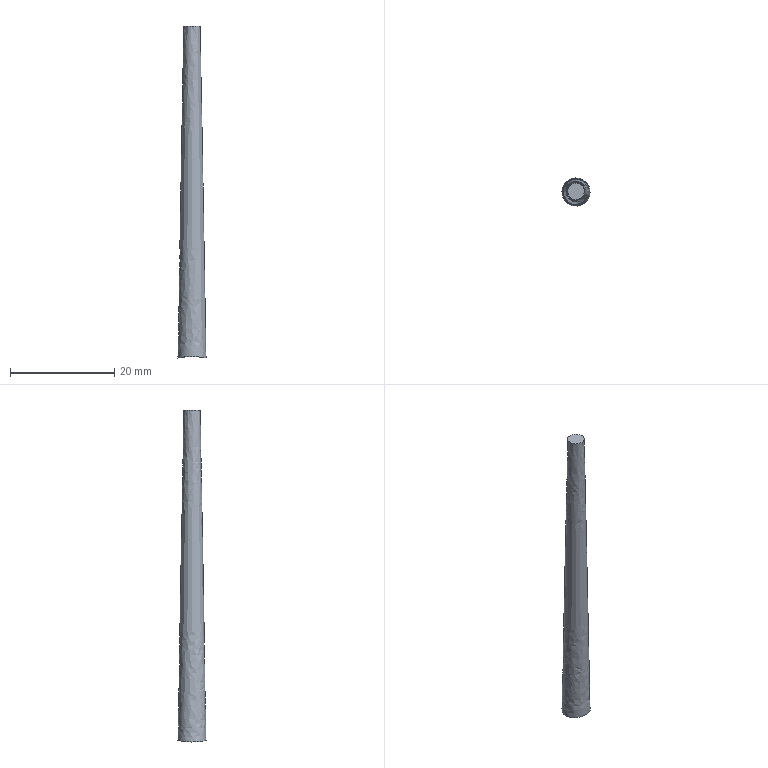Part | NX | features solid 2 | 1 solid | 3 faces | box 5.395 x 5.397 x 63.732 mm | volume 937.54 mm3 | spline 1 | plane 1 | cylinder 1 | commonest cylinder face diameters 26.633 x1